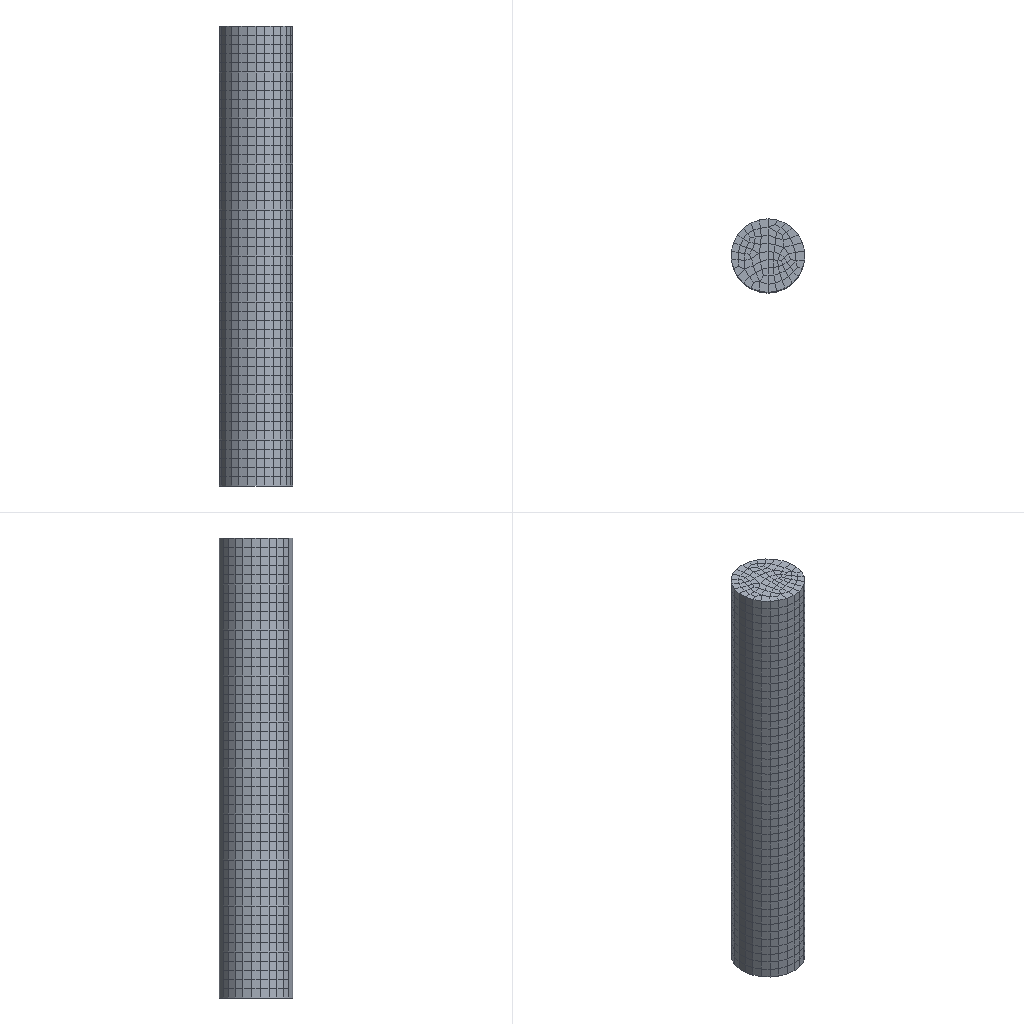Simulation study | abaqus
Set-up summary:
category,name,step,type,value,unit,region
solver,abaqus,,Abaqus/CAE 2024
units,mm-N-s-tonne (MPa),,inferred,E=100 density=1e-09
analysis,Step-1,,coupled temp-displacement,nlgeom=True; time_period=1
mesh,nodes,,,4998
mesh,elements,,,4200
element_type,C3D8T,,,4200
material,Material-1,,E,100
material,Material-1,,nu,0.45
material,Material-1,,density,1e-09
material,Material-1,,conductivity,10
material,Material-1,,specific_heat,1e+08
material,Material-1,,cte,-0.002
material,Material-1,,behaviors,conductivity; expansion; specific heat
material,Material-1-Copy,,E,2
material,Material-1-Copy,,nu,0.45
material,Material-1-Copy,,density,1e-09
material,Material-1-Copy,,conductivity,10
material,Material-1-Copy,,specific_heat,1e+08
material,Material-1-Copy,,cte,8e-05
material,Material-1-Copy,,behaviors,conductivity; expansion; specific heat
section,Material-1-Copy,,solid section,,,_PickedSet6
section,Material-1,,solid section,,,_PickedSet5
load,Predefined,initial,initial condition temperature
bc,BC-2,Step-1,displacement,1 [dofs=temp],,_PickedSet10
bc,BC-3,Step-1,fixed,[dofs=rz],,_PickedSet11
Abaqus input file, long lists of numbers shortened:
*Heading
** Job name: deck Model name: Model-1
** Generated by: Abaqus/CAE 2024
*Preprint, echo=NO, model=NO, history=NO, contact=NO
**
** PARTS
**
*Part, name=Part-1
*Node
      1,           0., 0.004,           0.
      2,           0., -0.004,           0.
** (4996 more lines like these left out)
*Element, type=C3D8T
   1,   23,  167,  188,   24,  824, 1863, 1884,  823
   2,  167,  170,  183,  194, 1863, 1866, 1879, 1890
** (4198 more lines like these left out)
*Nset, nset=_PickedSet5, internal
    1,    2,    3,    4,   17,   18,   19,   20,   21,   22,   23,   24,   25,   26,   27,   28
   29,   30,   31,   32,   33,   34,   35,   36,   37,   38,   39,   40,   41,   42,   43,   44
** (164 more lines like these left out)
*Elset, elset=_PickedSet5, internal, generate
 2201,  4200,     1
*Nset, nset=_PickedSet6, internal
    1,    2,    3,    4,    5,    6,    7,    8,    9,   10,   11,   12,   13,   14,   15,   16
   17,   18,   19,   20,   21,   22,   23,   24,   25,   26,   27,   28,   29,   30,   31,   32
** (177 more lines like these left out)
*Elset, elset=_PickedSet6, internal, generate
    1,  2200,     1
** Section: Section-2
*Solid Section, elset=_PickedSet6, material=Material-1-Copy
,
** Section: pin
*Solid Section, elset=_PickedSet5, material=Material-1
,
*End Part
**
**
** ASSEMBLY
**
*Assembly, name=Assembly
**
*Instance, name=Part-1-1, part=Part-1
*End Instance
**
*Nset, nset=_PickedSet8, internal, instance=Part-1-1, generate
    1,  4998,     1
*Elset, elset=_PickedSet8, internal, instance=Part-1-1, generate
    1,  4200,     1
*Nset, nset=_PickedSet9, internal, instance=Part-1-1
    3,    4,  123,  124,  125,  126,  127,  128,  129,  130,  131,  132,  133,  134,  135,  136
  137,  138,  139,  140,  141,  142,  155,  156,  157,  158,  159,  160,  161,  162,  163,  164
** (5 more lines like these left out)
*Elset, elset=_PickedSet9, internal, instance=Part-1-1
 2157, 2158, 2159, 2160, 2161, 2162, 2163, 2164, 2165, 2166, 2167, 2168, 2169, 2170, 2171, 2172
 2173, 2174, 2175, 2176, 2177, 2178, 2179, 2180, 2181, 2182, 2183, 2184, 2185, 2186, 2187, 2188
** (4 more lines like these left out)
*Nset, nset=_PickedSet10, internal, instance=Part-1-1
    1,    2,    3,    4,    5,    6,    7,    8,    9,   10,   11,   12,   13,   14,   15,   16
   25,   26,   27,   28,   29,   30,   31,   32,   33,   34,   35,   36,   37,   38,   39,   40
** (81 more lines like these left out)
*Elset, elset=_PickedSet10, internal, instance=Part-1-1
    6,    7,   12,   19,   21,   22,   24,   26,   27,   30,   31,   32,   38,   50,   51,   56
   63,   65,   66,   68,   70,   71,   74,   75,   76,   82,   94,   95,  100,  107,  109,  110
** (80 more lines like these left out)
*Nset, nset=_PickedSet11, internal, instance=Part-1-1
    3,    4,  123,  124,  125,  126,  127,  128,  129,  130,  131,  132,  133,  134,  135,  136
  137,  138,  139,  140,  141,  142,  155,  156,  157,  158,  159,  160,  161,  162,  163,  164
** (5 more lines like these left out)
*Elset, elset=_PickedSet11, internal, instance=Part-1-1
 2157, 2158, 2159, 2160, 2161, 2162, 2163, 2164, 2165, 2166, 2167, 2168, 2169, 2170, 2171, 2172
 2173, 2174, 2175, 2176, 2177, 2178, 2179, 2180, 2181, 2182, 2183, 2184, 2185, 2186, 2187, 2188
** (4 more lines like these left out)
*End Assembly
*Amplitude, name=Amp-1
             0.,             20.,              1.,             50.
*Amplitude, name=Amp-2
             0.,             32.,             0.5,             50.,              1.,             20.
**
** MATERIALS
**
*Material, name=Material-1
*Conductivity
10.,
*Density
 1e-09,
*Elastic
100., 0.45,  20.
100., 0.45,  32.
100., 0.45,  35.
100., 0.45,  40.
*Expansion
 -0.002,20.
     0.,32.
  0.002,50.
*Specific Heat
 1e+08,
*Material, name=Material-1-Copy
*Conductivity
10.,
*Density
 1e-09,
*Elastic
   2., 0.45,  20.
  1.5, 0.45,  40.
 0.25, 0.45,  60.
*Expansion
 8e-05,
*Specific Heat
 1e+08,
**
** PREDEFINED FIELDS
**
** Name: Predefined Field-1   Type: Temperature
*Initial Conditions, type=TEMPERATURE
_PickedSet8, 32.
** ----------------------------------------------------------------
**
** STEP: Step-1
**
*Step, name=Step-1, nlgeom=YES, inc=10000
*Coupled Temperature-displacement, creep=none, deltmx=10., stabilize=0.0002, allsdtol=0.05, continue=NO
0.01, 1., 1e-05, 0.1
**
** BOUNDARY CONDITIONS
**
** Name: BC-2 Type: Temperature
*Boundary, amplitude=Amp-2
_PickedSet10, 11, 11, 1.
** Name: BC-3 Type: Displacement/Rotation
*Boundary
_PickedSet11, 6, 6
**
** OUTPUT REQUESTS
**
*Restart, write, frequency=0
**
** FIELD OUTPUT: F-Output-1
**
*Output, field, variable=PRESELECT
**
** HISTORY OUTPUT: H-Output-1
**
*Output, history, variable=PRESELECT
*End Step
Results summary:
result,odb.job_status,,,JOB_STATUS_COMPLETED_SUCCESSFULLY,"consistent, unstated (Abaqus has no unit system)"
result,steps[0].procedure,Step-1,,"*COUPLED TEMPERATURE-DISPLACEMENT, STEADY STATE","consistent, unstated (Abaqus has no unit system)"
result,steps[0].time_period,Step-1,,1,"consistent, unstated (Abaqus has no unit system)"
result,steps[0].n_frames,Step-1,,16,"consistent, unstated (Abaqus has no unit system)"
result,steps[0].last_frame.id,Step-1,,15,"consistent, unstated (Abaqus has no unit system)"
result,steps[0].last_frame.value,Step-1,,1,"consistent, unstated (Abaqus has no unit system)"
result,steps[0].last_frame.description,Step-1,,Increment     15: Step Time =    1.000,"consistent, unstated (Abaqus has no unit system)"
result,steps[0].completed,Step-1,,True,"consistent, unstated (Abaqus has no unit system)"
result,steps[0].max_U_magnitude,Step-1,,0.001121,"consistent, unstated (Abaqus has no unit system)"
result,steps[0].max_S_mises,Step-1,,0.4925,"consistent, unstated (Abaqus has no unit system)"
result,steps[0].RF_sum[1],Step-1,,0,"consistent, unstated (Abaqus has no unit system)"
result,steps[0].RF_sum[2],Step-1,,0,"consistent, unstated (Abaqus has no unit system)"
result,steps[0].RF_sum[3],Step-1,,0,"consistent, unstated (Abaqus has no unit system)"